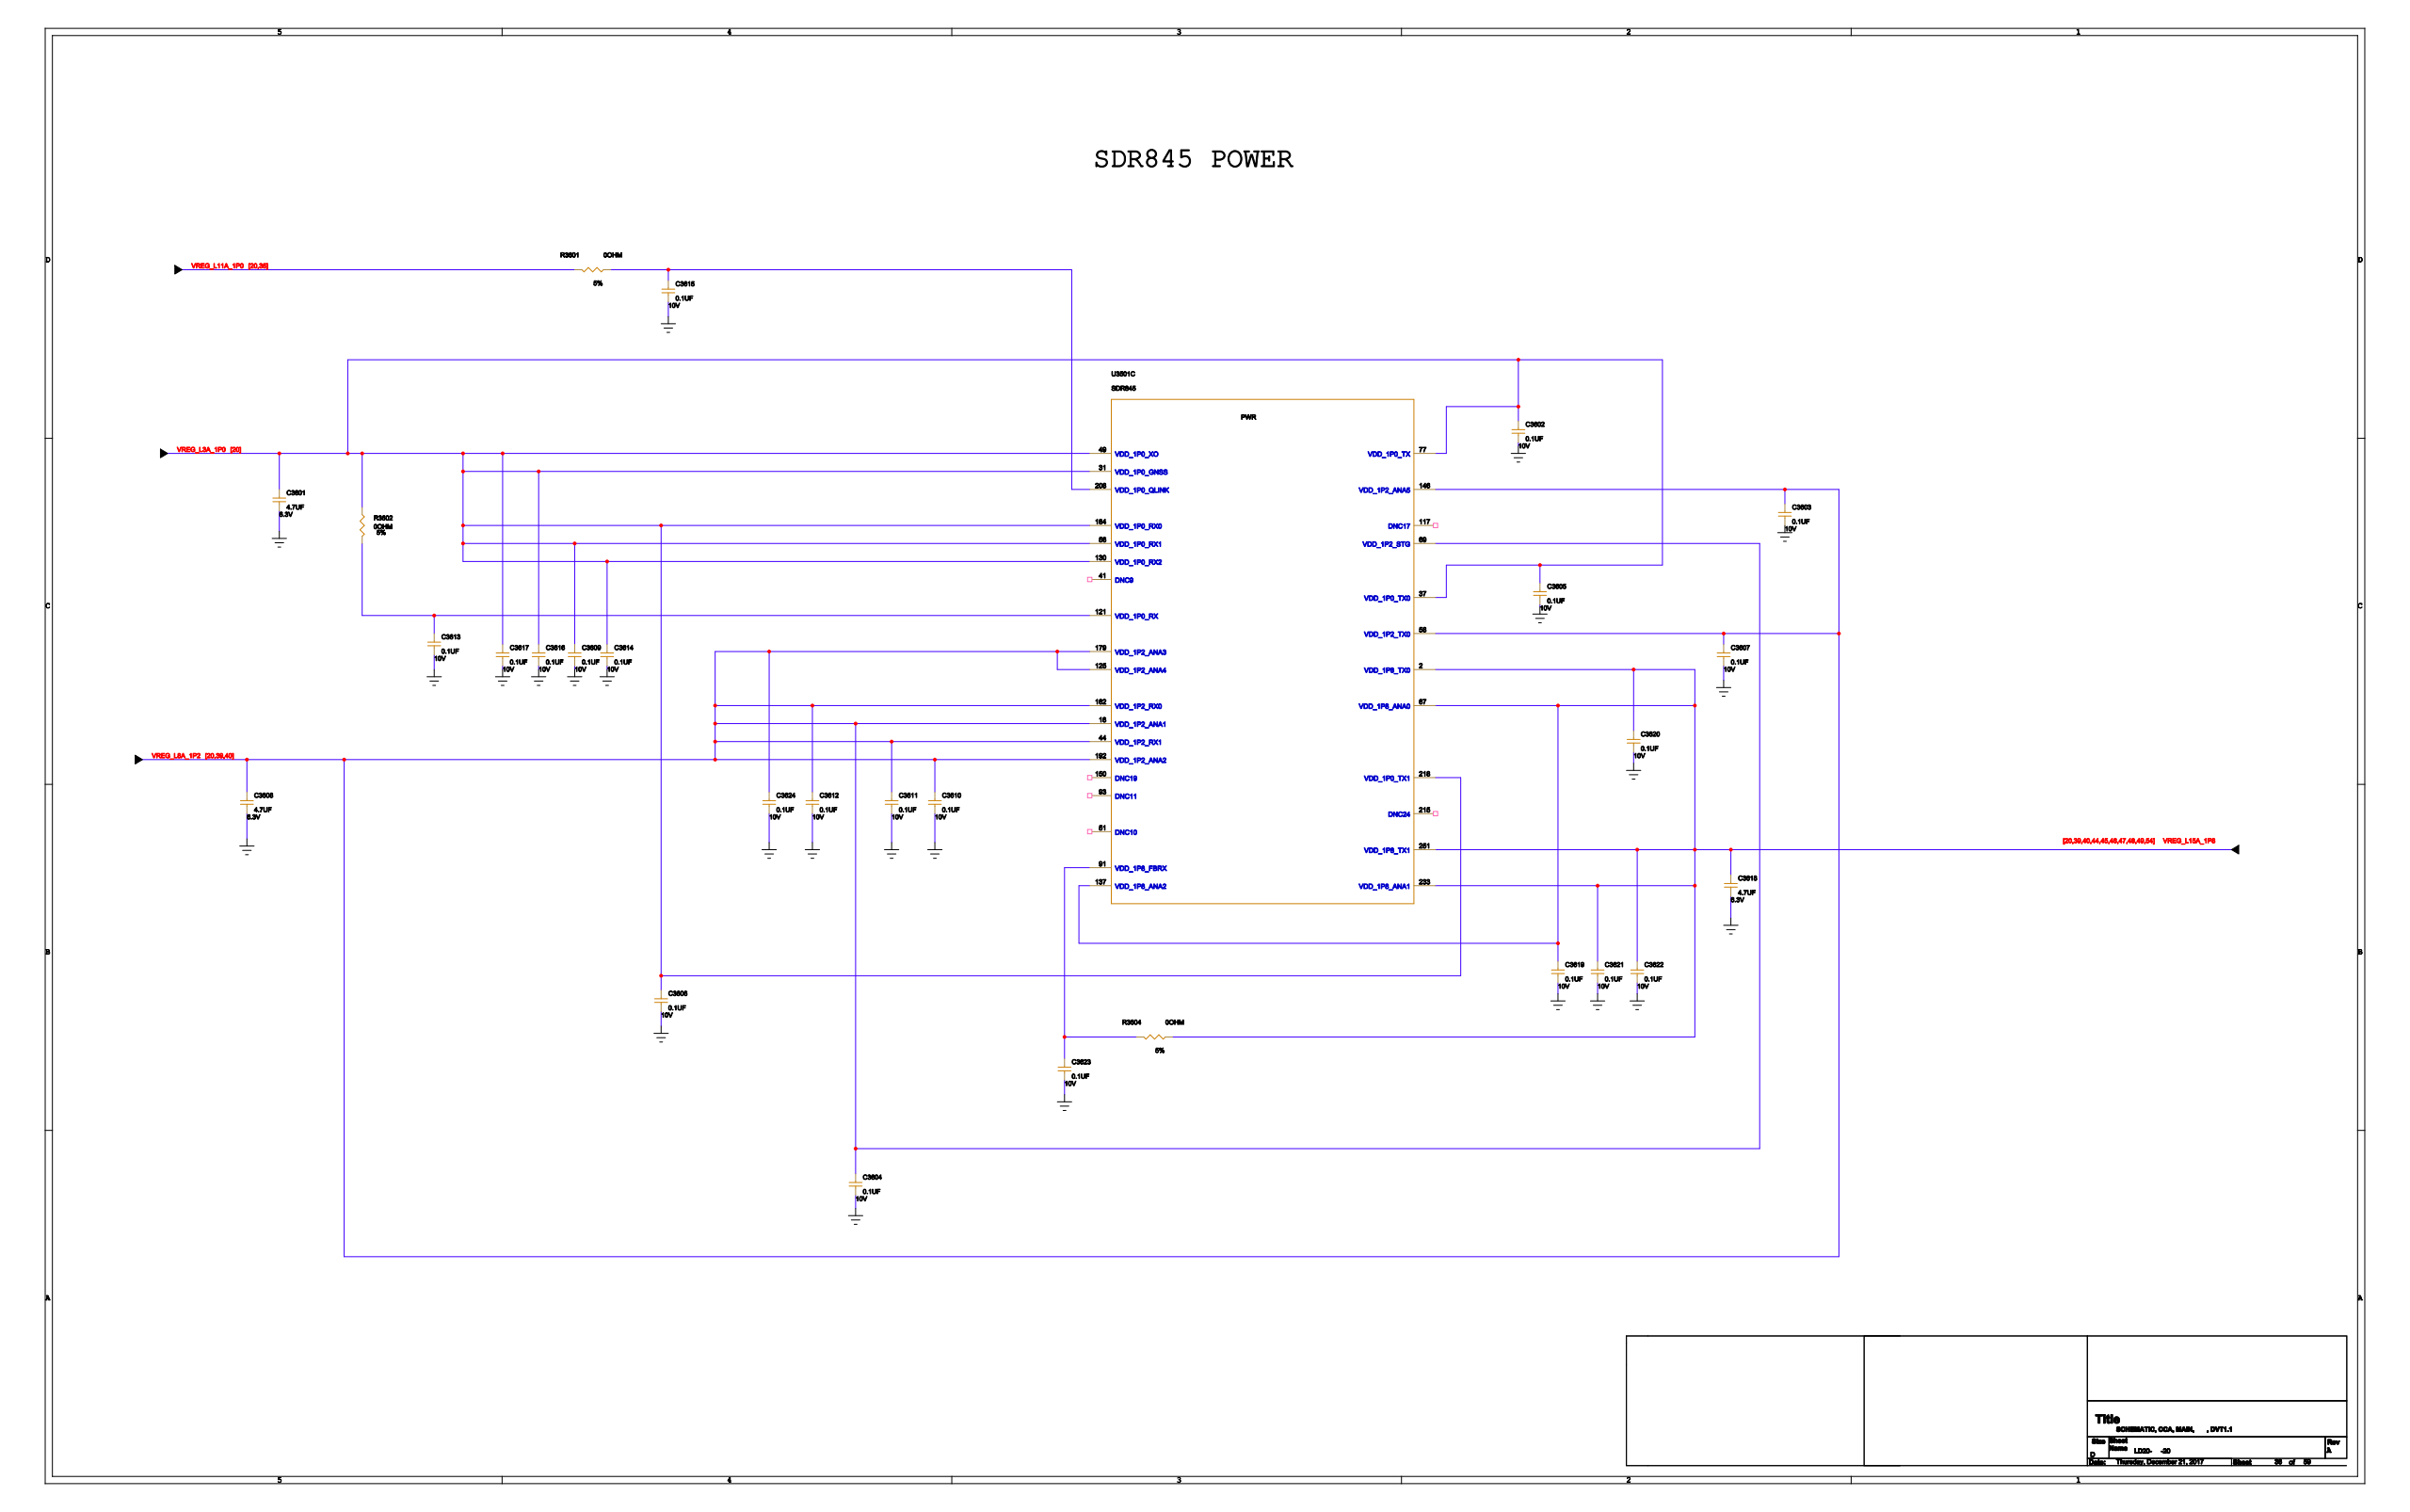Circuit board | Cadence Allegro | 1520 parts | 1149 nets | one sheet of the schematic
Parts on this sheet (reference | value | footprint):
C3601 | 4.7UF | 2P0402R
C3602 | 0.1UF | 2P0201R
C3603 | 0.1UF | 2P0201R
C3604 | 0.1UF | 2P0201R
C3605 | 0.1UF | 2P0201R
C3606 | 0.1UF | 2P0201R
C3607 | 0.1UF | 2P0201R
C3608 | 4.7UF | 2P0402R
C3609 | 0.1UF | 2P0201R
C3610 | 0.1UF | 2P0201R
C3611 | 0.1UF | 2P0201R
C3612 | 0.1UF | 2P0201R
C3613 | 0.1UF | 2P0201R
C3614 | 0.1UF | 2P0201R
C3615 | 0.1UF | 2P0201R
C3616 | 0.1UF | 2P0201R
C3617 | 0.1UF | 2P0201R
C3618 | 4.7UF | 2P0402R
C3619 | 0.1UF | 2P0201R
C3620 | 0.1UF | 2P0201R
C3621 | 0.1UF | 2P0201R
C3622 | 0.1UF | 2P0201R
C3623 | 0.1UF | 2P0201R
C3624 | 0.1UF | 2P0201R
R3601 | 0OHM | 2P0201R
R3602 | 0OHM | 2P0201R
R3604 | 0OHM | 2P0201R
U3501 | SDR845 | 253PGA235X247B138D45
Nets of these parts (net: part-pin ...):
GND: C3601-2 C3602-2 C3603-2 C3604-2 C3605-2 C3606-2 C3607-2 C3608-2 C3609-2 C3610-2 C3611-2 C3612-2 C3613-2 C3614-2 C3615-2 C3616-2 C3617-2 C3618-2 C3619-2 C3620-2 C3621-2 C3622-2 C3623-2 C3624-2 U3501-5 U3501-21 U3501-36 U3501-39 U3501-40 U3501-45 U3501-46 U3501-47 U3501-48 U3501-59
VREG_L15A_1P8: C3618-1 C3619-1 C3620-1 C3621-1 C3622-1 R3604-2 U3501-2 U3501-67 U3501-137 U3501-233 U3501-251
VREG_L11A_1P0: R3601-1
VREG_L3A_1P0: C3601-1 C3602-1 C3605-1 C3606-1 C3609-1 C3614-1 C3616-1 C3617-1 R3602-2 U3501-31 U3501-37 U3501-49 U3501-56 U3501-77 U3501-130 U3501-184 U3501-218
N33733482: C3615-1 R3601-2 U3501-208
N33733594: C3613-1 R3602-1 U3501-121
VREG_L8A_1P2: C3603-1 C3604-1 C3607-1 C3608-1 C3610-1 C3611-1 C3612-1 C3624-1 U3501-18 U3501-44 U3501-58 U3501-69 U3501-125 U3501-146 U3501-162 U3501-179 U3501-192
N33735828: C3623-1 R3604-1 U3501-91